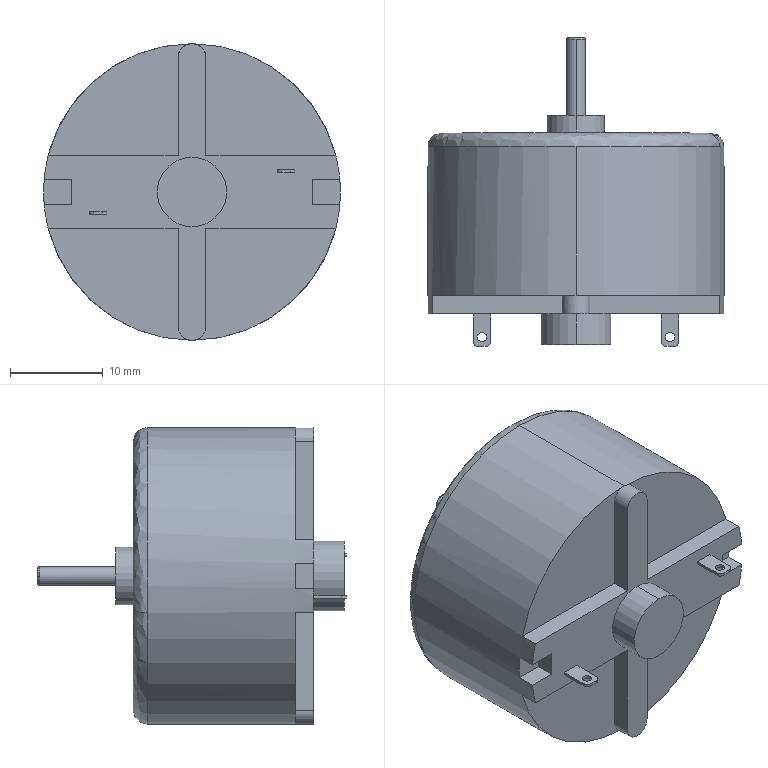Part | SolidWorks | features ICE 2, BaseBody 1, MoveFace 1 | 1 solid | 64 faces | box 32 x 33.3 x 32 mm | volume 14832 mm3 | plane 37 | cylinder 23 | spline 4 | commonest cylinder face diameters 1 x8 2.6 x4 3 x3 2 x2 6.2 x2 7.5 x2